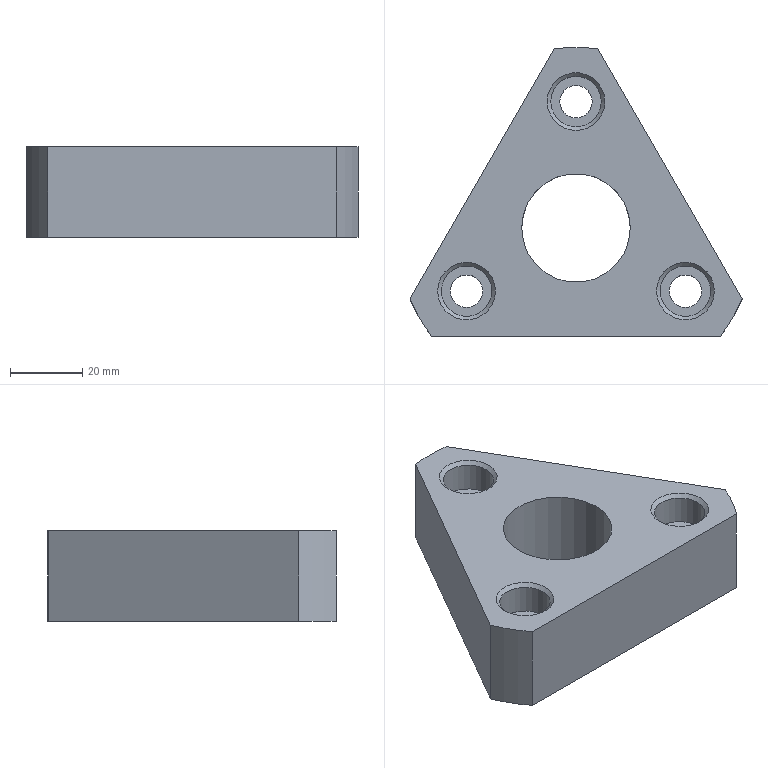Part | NX | 1 solid | 21 faces | box 91.962 x 80 x 25 mm | volume 87413 mm3 | cylinder 10 | plane 8 | cone 3 | commonest cylinder face diameters 9 x3 14 x3 100 x3 30.1 x1
STEP:
#1=CARTESIAN_POINT('',(-4.5,25.,-25.));
#2=VERTEX_POINT('',#1);
#3=CARTESIAN_POINT('',(0.,25.,-25.));
#4=DIRECTION('',(0.,0.,1.));
#5=DIRECTION('',(-1.,0.,0.));
#6=AXIS2_PLACEMENT_3D('',#3,#4,#5);
#7=CIRCLE('',#6,4.5);
#8=EDGE_CURVE('',#2,#2,#7,.T.);
#9=ORIENTED_EDGE('',*,*,#8,.F.);
#10=EDGE_LOOP('',(#9));
#11=FACE_BOUND('',#10,.T.);
#12=CARTESIAN_POINT('',(-4.5,25.,-9.));
#13=VERTEX_POINT('',#12);
#14=CARTESIAN_POINT('',(0.,25.,-9.));
#15=DIRECTION('',(0.,0.,1.));
#16=DIRECTION('',(-1.,0.,0.));
#17=AXIS2_PLACEMENT_3D('',#14,#15,#16);
#18=CIRCLE('',#17,4.5);
#19=EDGE_CURVE('',#13,#13,#18,.F.);
#20=ORIENTED_EDGE('',*,*,#19,.F.);
#21=EDGE_LOOP('',(#20));
#22=FACE_BOUND('',#21,.T.);
#23=CARTESIAN_POINT('',(0.,25.,-25.));
#24=DIRECTION('',(0.,0.,1.));
#25=DIRECTION('',(-1.,0.,0.));
#26=AXIS2_PLACEMENT_3D('',#23,#24,#25);
#27=CYLINDRICAL_SURFACE('',#26,4.5);
#28=ADVANCED_FACE('',(#11,#22),#27,.F.);
#29=CARTESIAN_POINT('',(-34.811,-27.5,-25.));
#30=VERTEX_POINT('',#29);
#31=CARTESIAN_POINT('',(-30.311,-27.5,-25.));
#32=DIRECTION('',(0.,0.,1.));
#33=DIRECTION('',(-1.,0.,0.));
#34=AXIS2_PLACEMENT_3D('',#31,#32,#33);
#35=CIRCLE('',#34,4.5);
#36=EDGE_CURVE('',#30,#30,#35,.T.);
#37=ORIENTED_EDGE('',*,*,#36,.F.);
#38=EDGE_LOOP('',(#37));
#39=FACE_BOUND('',#38,.T.);
#40=CARTESIAN_POINT('',(-34.811,-27.5,-9.));
#41=VERTEX_POINT('',#40);
#42=CARTESIAN_POINT('',(-30.311,-27.5,-9.));
#43=DIRECTION('',(0.,0.,1.));
#44=DIRECTION('',(-1.,0.,0.));
#45=AXIS2_PLACEMENT_3D('',#42,#43,#44);
#46=CIRCLE('',#45,4.5);
#47=EDGE_CURVE('',#41,#41,#46,.F.);
#48=ORIENTED_EDGE('',*,*,#47,.F.);
#49=EDGE_LOOP('',(#48));
#50=FACE_BOUND('',#49,.T.);
#51=CARTESIAN_POINT('',(-30.311,-27.5,-25.));
#52=DIRECTION('',(0.,0.,1.));
#53=DIRECTION('',(-1.,0.,0.));
#54=AXIS2_PLACEMENT_3D('',#51,#52,#53);
#55=CYLINDRICAL_SURFACE('',#54,4.5);
#56=ADVANCED_FACE('',(#39,#50),#55,.F.);
#57=CARTESIAN_POINT('',(25.811,-27.5,-25.));
#58=VERTEX_POINT('',#57);
#59=CARTESIAN_POINT('',(30.311,-27.5,-25.));
#60=DIRECTION('',(0.,0.,1.));
#61=DIRECTION('',(-1.,0.,0.));
#62=AXIS2_PLACEMENT_3D('',#59,#60,#61);
#63=CIRCLE('',#62,4.5);
#64=EDGE_CURVE('',#58,#58,#63,.T.);
#65=ORIENTED_EDGE('',*,*,#64,.F.);
#66=EDGE_LOOP('',(#65));
#67=FACE_BOUND('',#66,.T.);
#68=CARTESIAN_POINT('',(25.811,-27.5,-9.));
#69=VERTEX_POINT('',#68);
#70=CARTESIAN_POINT('',(30.311,-27.5,-9.));
#71=DIRECTION('',(0.,0.,1.));
#72=DIRECTION('',(-1.,0.,0.));
#73=AXIS2_PLACEMENT_3D('',#70,#71,#72);
#74=CIRCLE('',#73,4.5);
#75=EDGE_CURVE('',#69,#69,#74,.F.);
#76=ORIENTED_EDGE('',*,*,#75,.F.);
#77=EDGE_LOOP('',(#76));
#78=FACE_BOUND('',#77,.T.);
#79=CARTESIAN_POINT('',(30.311,-27.5,-25.));
#80=DIRECTION('',(0.,0.,1.));
#81=DIRECTION('',(-1.,0.,0.));
#82=AXIS2_PLACEMENT_3D('',#79,#80,#81);
#83=CYLINDRICAL_SURFACE('',#82,4.5);
#84=ADVANCED_FACE('',(#67,#78),#83,.F.);
#85=CARTESIAN_POINT('',(40.,-40.,0.));
#86=VERTEX_POINT('',#85);
#87=CARTESIAN_POINT('',(-40.,-40.,0.));
#88=VERTEX_POINT('',#87);
#89=CARTESIAN_POINT('',(40.,-40.,0.));
#90=DIRECTION('',(-1.,0.,0.));
#91=VECTOR('',#90,1000.);
#92=LINE('',#89,#91);
#93=EDGE_CURVE('',#86,#88,#92,.T.);
#94=ORIENTED_EDGE('',*,*,#93,.T.);
#95=CARTESIAN_POINT('',(-40.,-40.,-25.));
#96=VERTEX_POINT('',#95);
#97=CARTESIAN_POINT('',(-40.,-40.,-25.));
#98=DIRECTION('',(0.,0.,1.));
#99=VECTOR('',#98,1000.);
#100=LINE('',#97,#99);
#101=EDGE_CURVE('',#96,#88,#100,.T.);
#102=ORIENTED_EDGE('',*,*,#101,.F.);
#103=CARTESIAN_POINT('',(40.,-40.,-25.));
#104=VERTEX_POINT('',#103);
#105=CARTESIAN_POINT('',(40.,-40.,-25.));
#106=DIRECTION('',(-1.,0.,0.));
#107=VECTOR('',#106,1000.);
#108=LINE('',#105,#107);
#109=EDGE_CURVE('',#104,#96,#108,.T.);
#110=ORIENTED_EDGE('',*,*,#109,.F.);
#111=CARTESIAN_POINT('',(40.,-40.,-25.));
#112=DIRECTION('',(0.,0.,1.));
#113=VECTOR('',#112,1000.);
#114=LINE('',#111,#113);
#115=EDGE_CURVE('',#104,#86,#114,.T.);
#116=ORIENTED_EDGE('',*,*,#115,.T.);
#117=EDGE_LOOP('',(#94,#102,#110,#116));
#118=FACE_BOUND('',#117,.T.);
#119=CARTESIAN_POINT('',(40.,-40.,-25.));
#120=DIRECTION('',(0.,1.,0.));
#121=DIRECTION('',(-1.,0.,0.));
#122=AXIS2_PLACEMENT_3D('',#119,#120,#121);
#123=PLANE('',#122);
#124=ADVANCED_FACE('',(#118),#123,.F.);
#125=CARTESIAN_POINT('',(-45.981,-29.641,0.));
#126=VERTEX_POINT('',#125);
#127=CARTESIAN_POINT('',(0.,-10.,0.));
#128=DIRECTION('',(0.,0.,-1.));
#129=DIRECTION('',(-1.,0.,0.));
#130=AXIS2_PLACEMENT_3D('',#127,#128,#129);
#131=CIRCLE('',#130,50.);
#132=EDGE_CURVE('',#88,#126,#131,.T.);
#133=ORIENTED_EDGE('',*,*,#132,.T.);
#134=CARTESIAN_POINT('',(-45.981,-29.641,-25.));
#135=VERTEX_POINT('',#134);
#136=CARTESIAN_POINT('',(-45.981,-29.641,-25.));
#137=DIRECTION('',(0.,0.,1.));
#138=VECTOR('',#137,1000.);
#139=LINE('',#136,#138);
#140=EDGE_CURVE('',#135,#126,#139,.T.);
#141=ORIENTED_EDGE('',*,*,#140,.F.);
#142=CARTESIAN_POINT('',(0.,-10.,-25.));
#143=DIRECTION('',(0.,0.,-1.));
#144=DIRECTION('',(-1.,0.,0.));
#145=AXIS2_PLACEMENT_3D('',#142,#143,#144);
#146=CIRCLE('',#145,50.);
#147=EDGE_CURVE('',#96,#135,#146,.T.);
#148=ORIENTED_EDGE('',*,*,#147,.F.);
#149=ORIENTED_EDGE('',*,*,#101,.T.);
#150=EDGE_LOOP('',(#133,#141,#148,#149));
#151=FACE_BOUND('',#150,.T.);
#152=CARTESIAN_POINT('',(0.,-10.,-25.));
#153=DIRECTION('',(0.,0.,1.));
#154=DIRECTION('',(-1.,0.,0.));
#155=AXIS2_PLACEMENT_3D('',#152,#153,#154);
#156=CYLINDRICAL_SURFACE('',#155,50.);
#157=ADVANCED_FACE('',(#151),#156,.T.);
#158=CARTESIAN_POINT('',(-5.981,39.641,0.));
#159=VERTEX_POINT('',#158);
#160=CARTESIAN_POINT('',(-45.981,-29.641,0.));
#161=DIRECTION('',(0.5,0.866,0.));
#162=VECTOR('',#161,1000.);
#163=LINE('',#160,#162);
#164=EDGE_CURVE('',#126,#159,#163,.T.);
#165=ORIENTED_EDGE('',*,*,#164,.T.);
#166=CARTESIAN_POINT('',(-5.981,39.641,-25.));
#167=VERTEX_POINT('',#166);
#168=CARTESIAN_POINT('',(-5.981,39.641,-25.));
#169=DIRECTION('',(0.,0.,1.));
#170=VECTOR('',#169,1000.);
#171=LINE('',#168,#170);
#172=EDGE_CURVE('',#167,#159,#171,.T.);
#173=ORIENTED_EDGE('',*,*,#172,.F.);
#174=CARTESIAN_POINT('',(-45.981,-29.641,-25.));
#175=DIRECTION('',(0.5,0.866,0.));
#176=VECTOR('',#175,1000.);
#177=LINE('',#174,#176);
#178=EDGE_CURVE('',#135,#167,#177,.T.);
#179=ORIENTED_EDGE('',*,*,#178,.F.);
#180=ORIENTED_EDGE('',*,*,#140,.T.);
#181=EDGE_LOOP('',(#165,#173,#179,#180));
#182=FACE_BOUND('',#181,.T.);
#183=CARTESIAN_POINT('',(-45.981,-29.641,-25.));
#184=DIRECTION('',(0.866,-0.5,0.));
#185=DIRECTION('',(0.5,0.866,0.));
#186=AXIS2_PLACEMENT_3D('',#183,#184,#185);
#187=PLANE('',#186);
#188=ADVANCED_FACE('',(#182),#187,.F.);
#189=CARTESIAN_POINT('',(5.981,39.641,0.));
#190=VERTEX_POINT('',#189);
#191=CARTESIAN_POINT('',(0.,-10.,0.));
#192=DIRECTION('',(0.,0.,-1.));
#193=DIRECTION('',(-1.,0.,0.));
#194=AXIS2_PLACEMENT_3D('',#191,#192,#193);
#195=CIRCLE('',#194,50.);
#196=EDGE_CURVE('',#159,#190,#195,.T.);
#197=ORIENTED_EDGE('',*,*,#196,.T.);
#198=CARTESIAN_POINT('',(5.981,39.641,-25.));
#199=VERTEX_POINT('',#198);
#200=CARTESIAN_POINT('',(5.981,39.641,-25.));
#201=DIRECTION('',(0.,0.,1.));
#202=VECTOR('',#201,1000.);
#203=LINE('',#200,#202);
#204=EDGE_CURVE('',#199,#190,#203,.T.);
#205=ORIENTED_EDGE('',*,*,#204,.F.);
#206=CARTESIAN_POINT('',(0.,-10.,-25.));
#207=DIRECTION('',(0.,0.,-1.));
#208=DIRECTION('',(-1.,0.,0.));
#209=AXIS2_PLACEMENT_3D('',#206,#207,#208);
#210=CIRCLE('',#209,50.);
#211=EDGE_CURVE('',#167,#199,#210,.T.);
#212=ORIENTED_EDGE('',*,*,#211,.F.);
#213=ORIENTED_EDGE('',*,*,#172,.T.);
#214=EDGE_LOOP('',(#197,#205,#212,#213));
#215=FACE_BOUND('',#214,.T.);
#216=CARTESIAN_POINT('',(0.,-10.,-25.));
#217=DIRECTION('',(0.,0.,1.));
#218=DIRECTION('',(-1.,0.,0.));
#219=AXIS2_PLACEMENT_3D('',#216,#217,#218);
#220=CYLINDRICAL_SURFACE('',#219,50.);
#221=ADVANCED_FACE('',(#215),#220,.T.);
#222=CARTESIAN_POINT('',(45.981,-29.641,0.));
#223=VERTEX_POINT('',#222);
#224=CARTESIAN_POINT('',(5.981,39.641,0.));
#225=DIRECTION('',(0.5,-0.866,0.));
#226=VECTOR('',#225,1000.);
#227=LINE('',#224,#226);
#228=EDGE_CURVE('',#190,#223,#227,.T.);
#229=ORIENTED_EDGE('',*,*,#228,.T.);
#230=CARTESIAN_POINT('',(45.981,-29.641,-25.));
#231=VERTEX_POINT('',#230);
#232=CARTESIAN_POINT('',(45.981,-29.641,-25.));
#233=DIRECTION('',(0.,0.,1.));
#234=VECTOR('',#233,1000.);
#235=LINE('',#232,#234);
#236=EDGE_CURVE('',#231,#223,#235,.T.);
#237=ORIENTED_EDGE('',*,*,#236,.F.);
#238=CARTESIAN_POINT('',(5.981,39.641,-25.));
#239=DIRECTION('',(0.5,-0.866,0.));
#240=VECTOR('',#239,1000.);
#241=LINE('',#238,#240);
#242=EDGE_CURVE('',#199,#231,#241,.T.);
#243=ORIENTED_EDGE('',*,*,#242,.F.);
#244=ORIENTED_EDGE('',*,*,#204,.T.);
#245=EDGE_LOOP('',(#229,#237,#243,#244));
#246=FACE_BOUND('',#245,.T.);
#247=CARTESIAN_POINT('',(5.981,39.641,-25.));
#248=DIRECTION('',(-0.866,-0.5,0.));
#249=DIRECTION('',(0.5,-0.866,0.));
#250=AXIS2_PLACEMENT_3D('',#247,#248,#249);
#251=PLANE('',#250);
#252=ADVANCED_FACE('',(#246),#251,.F.);
#253=CARTESIAN_POINT('',(15.05,-10.,-25.));
#254=VERTEX_POINT('',#253);
#255=CARTESIAN_POINT('',(0.,-10.,-25.));
#256=DIRECTION('',(0.,0.,-1.));
#257=DIRECTION('',(1.,0.,0.));
#258=AXIS2_PLACEMENT_3D('',#255,#256,#257);
#259=CIRCLE('',#258,15.05);
#260=EDGE_CURVE('',#254,#254,#259,.F.);
#261=ORIENTED_EDGE('',*,*,#260,.F.);
#262=EDGE_LOOP('',(#261));
#263=FACE_BOUND('',#262,.T.);
#264=CARTESIAN_POINT('',(15.05,-10.,0.));
#265=VERTEX_POINT('',#264);
#266=CARTESIAN_POINT('',(0.,-10.,0.));
#267=DIRECTION('',(0.,0.,-1.));
#268=DIRECTION('',(1.,0.,0.));
#269=AXIS2_PLACEMENT_3D('',#266,#267,#268);
#270=CIRCLE('',#269,15.05);
#271=EDGE_CURVE('',#265,#265,#270,.F.);
#272=ORIENTED_EDGE('',*,*,#271,.T.);
#273=EDGE_LOOP('',(#272));
#274=FACE_BOUND('',#273,.T.);
#275=CARTESIAN_POINT('',(0.,-10.,-25.));
#276=DIRECTION('',(0.,0.,1.));
#277=DIRECTION('',(-1.,0.,0.));
#278=AXIS2_PLACEMENT_3D('',#275,#276,#277);
#279=CYLINDRICAL_SURFACE('',#278,15.05);
#280=ADVANCED_FACE('',(#263,#274),#279,.F.);
#281=CARTESIAN_POINT('',(0.,-10.,0.));
#282=DIRECTION('',(0.,0.,-1.));
#283=DIRECTION('',(-1.,0.,0.));
#284=AXIS2_PLACEMENT_3D('',#281,#282,#283);
#285=CIRCLE('',#284,50.);
#286=EDGE_CURVE('',#223,#86,#285,.T.);
#287=ORIENTED_EDGE('',*,*,#286,.T.);
#288=ORIENTED_EDGE('',*,*,#115,.F.);
#289=CARTESIAN_POINT('',(0.,-10.,-25.));
#290=DIRECTION('',(0.,0.,-1.));
#291=DIRECTION('',(-1.,0.,0.));
#292=AXIS2_PLACEMENT_3D('',#289,#290,#291);
#293=CIRCLE('',#292,50.);
#294=EDGE_CURVE('',#231,#104,#293,.T.);
#295=ORIENTED_EDGE('',*,*,#294,.F.);
#296=ORIENTED_EDGE('',*,*,#236,.T.);
#297=EDGE_LOOP('',(#287,#288,#295,#296));
#298=FACE_BOUND('',#297,.T.);
#299=CARTESIAN_POINT('',(0.,-10.,-25.));
#300=DIRECTION('',(0.,0.,1.));
#301=DIRECTION('',(-1.,0.,0.));
#302=AXIS2_PLACEMENT_3D('',#299,#300,#301);
#303=CYLINDRICAL_SURFACE('',#302,50.);
#304=ADVANCED_FACE('',(#298),#303,.T.);
#305=ORIENTED_EDGE('',*,*,#109,.T.);
#306=ORIENTED_EDGE('',*,*,#147,.T.);
#307=ORIENTED_EDGE('',*,*,#178,.T.);
#308=ORIENTED_EDGE('',*,*,#211,.T.);
#309=ORIENTED_EDGE('',*,*,#242,.T.);
#310=ORIENTED_EDGE('',*,*,#294,.T.);
#311=EDGE_LOOP('',(#305,#306,#307,#308,#309,#310));
#312=FACE_BOUND('',#311,.T.);
#313=ORIENTED_EDGE('',*,*,#36,.T.);
#314=EDGE_LOOP('',(#313));
#315=FACE_BOUND('',#314,.T.);
#316=ORIENTED_EDGE('',*,*,#8,.T.);
#317=EDGE_LOOP('',(#316));
#318=FACE_BOUND('',#317,.T.);
#319=ORIENTED_EDGE('',*,*,#260,.T.);
#320=EDGE_LOOP('',(#319));
#321=FACE_BOUND('',#320,.T.);
#322=ORIENTED_EDGE('',*,*,#64,.T.);
#323=EDGE_LOOP('',(#322));
#324=FACE_BOUND('',#323,.T.);
#325=CARTESIAN_POINT('',(0.,-10.,-25.));
#326=DIRECTION('',(0.,0.,-1.));
#327=DIRECTION('',(1.,0.,0.));
#328=AXIS2_PLACEMENT_3D('',#325,#326,#327);
#329=PLANE('',#328);
#330=ADVANCED_FACE('',(#312,#315,#318,#321,#324),#329,.T.);
#331=CARTESIAN_POINT('',(22.311,-27.5,0.));
#332=VERTEX_POINT('',#331);
#333=CARTESIAN_POINT('',(30.311,-27.5,0.));
#334=DIRECTION('',(0.,0.,-1.));
#335=DIRECTION('',(-1.,0.,0.));
#336=AXIS2_PLACEMENT_3D('',#333,#334,#335);
#337=CIRCLE('',#336,8.);
#338=EDGE_CURVE('',#332,#332,#337,.T.);
#339=ORIENTED_EDGE('',*,*,#338,.T.);
#340=EDGE_LOOP('',(#339));
#341=FACE_BOUND('',#340,.T.);
#342=CARTESIAN_POINT('',(-38.311,-27.5,0.));
#343=VERTEX_POINT('',#342);
#344=CARTESIAN_POINT('',(-30.311,-27.5,0.));
#345=DIRECTION('',(0.,0.,-1.));
#346=DIRECTION('',(-1.,0.,0.));
#347=AXIS2_PLACEMENT_3D('',#344,#345,#346);
#348=CIRCLE('',#347,8.);
#349=EDGE_CURVE('',#343,#343,#348,.T.);
#350=ORIENTED_EDGE('',*,*,#349,.T.);
#351=EDGE_LOOP('',(#350));
#352=FACE_BOUND('',#351,.T.);
#353=CARTESIAN_POINT('',(-8.,25.,0.));
#354=VERTEX_POINT('',#353);
#355=CARTESIAN_POINT('',(0.,25.,0.));
#356=DIRECTION('',(0.,0.,-1.));
#357=DIRECTION('',(-1.,0.,0.));
#358=AXIS2_PLACEMENT_3D('',#355,#356,#357);
#359=CIRCLE('',#358,8.);
#360=EDGE_CURVE('',#354,#354,#359,.T.);
#361=ORIENTED_EDGE('',*,*,#360,.T.);
#362=EDGE_LOOP('',(#361));
#363=FACE_BOUND('',#362,.T.);
#364=ORIENTED_EDGE('',*,*,#93,.F.);
#365=ORIENTED_EDGE('',*,*,#286,.F.);
#366=ORIENTED_EDGE('',*,*,#228,.F.);
#367=ORIENTED_EDGE('',*,*,#196,.F.);
#368=ORIENTED_EDGE('',*,*,#164,.F.);
#369=ORIENTED_EDGE('',*,*,#132,.F.);
#370=EDGE_LOOP('',(#364,#365,#366,#367,#368,#369));
#371=FACE_BOUND('',#370,.T.);
#372=ORIENTED_EDGE('',*,*,#271,.F.);
#373=EDGE_LOOP('',(#372));
#374=FACE_BOUND('',#373,.T.);
#375=CARTESIAN_POINT('',(0.,-10.,0.));
#376=DIRECTION('',(0.,0.,-1.));
#377=DIRECTION('',(1.,0.,0.));
#378=AXIS2_PLACEMENT_3D('',#375,#376,#377);
#379=PLANE('',#378);
#380=ADVANCED_FACE('',(#341,#352,#363,#371,#374),#379,.F.);
#381=CARTESIAN_POINT('',(23.311,-27.5,-9.));
#382=VERTEX_POINT('',#381);
#383=CARTESIAN_POINT('',(30.311,-27.5,-9.));
#384=DIRECTION('',(0.,0.,1.));
#385=DIRECTION('',(-1.,0.,0.));
#386=AXIS2_PLACEMENT_3D('',#383,#384,#385);
#387=CIRCLE('',#386,7.);
#388=EDGE_CURVE('',#382,#382,#387,.F.);
#389=ORIENTED_EDGE('',*,*,#388,.F.);
#390=EDGE_LOOP('',(#389));
#391=FACE_BOUND('',#390,.T.);
#392=ORIENTED_EDGE('',*,*,#75,.T.);
#393=EDGE_LOOP('',(#392));
#394=FACE_BOUND('',#393,.T.);
#395=CARTESIAN_POINT('',(30.311,-27.5,-9.));
#396=DIRECTION('',(0.,0.,1.));
#397=DIRECTION('',(-1.,0.,0.));
#398=AXIS2_PLACEMENT_3D('',#395,#396,#397);
#399=PLANE('',#398);
#400=ADVANCED_FACE('',(#391,#394),#399,.T.);
#401=CARTESIAN_POINT('',(23.311,-27.5,-1.));
#402=VERTEX_POINT('',#401);
#403=CARTESIAN_POINT('',(30.311,-27.5,-1.));
#404=DIRECTION('',(0.,0.,-1.));
#405=DIRECTION('',(-1.,0.,0.));
#406=AXIS2_PLACEMENT_3D('',#403,#404,#405);
#407=CIRCLE('',#406,7.);
#408=EDGE_CURVE('',#402,#402,#407,.F.);
#409=ORIENTED_EDGE('',*,*,#408,.T.);
#410=EDGE_LOOP('',(#409));
#411=FACE_BOUND('',#410,.T.);
#412=ORIENTED_EDGE('',*,*,#388,.T.);
#413=EDGE_LOOP('',(#412));
#414=FACE_BOUND('',#413,.T.);
#415=CARTESIAN_POINT('',(30.311,-27.5,-9.));
#416=DIRECTION('',(0.,0.,1.));
#417=DIRECTION('',(-1.,0.,0.));
#418=AXIS2_PLACEMENT_3D('',#415,#416,#417);
#419=CYLINDRICAL_SURFACE('',#418,7.);
#420=ADVANCED_FACE('',(#411,#414),#419,.F.);
#421=CARTESIAN_POINT('',(-7.,25.,-9.));
#422=VERTEX_POINT('',#421);
#423=CARTESIAN_POINT('',(0.,25.,-9.));
#424=DIRECTION('',(0.,0.,1.));
#425=DIRECTION('',(-1.,0.,0.));
#426=AXIS2_PLACEMENT_3D('',#423,#424,#425);
#427=CIRCLE('',#426,7.);
#428=EDGE_CURVE('',#422,#422,#427,.F.);
#429=ORIENTED_EDGE('',*,*,#428,.F.);
#430=EDGE_LOOP('',(#429));
#431=FACE_BOUND('',#430,.T.);
#432=ORIENTED_EDGE('',*,*,#19,.T.);
#433=EDGE_LOOP('',(#432));
#434=FACE_BOUND('',#433,.T.);
#435=CARTESIAN_POINT('',(0.,25.,-9.));
#436=DIRECTION('',(0.,0.,1.));
#437=DIRECTION('',(-1.,0.,0.));
#438=AXIS2_PLACEMENT_3D('',#435,#436,#437);
#439=PLANE('',#438);
#440=ADVANCED_FACE('',(#431,#434),#439,.T.);
#441=CARTESIAN_POINT('',(-7.,25.,-1.));
#442=VERTEX_POINT('',#441);
#443=CARTESIAN_POINT('',(0.,25.,-1.));
#444=DIRECTION('',(0.,0.,-1.));
#445=DIRECTION('',(-1.,0.,0.));
#446=AXIS2_PLACEMENT_3D('',#443,#444,#445);
#447=CIRCLE('',#446,7.);
#448=EDGE_CURVE('',#442,#442,#447,.F.);
#449=ORIENTED_EDGE('',*,*,#448,.T.);
#450=EDGE_LOOP('',(#449));
#451=FACE_BOUND('',#450,.T.);
#452=ORIENTED_EDGE('',*,*,#428,.T.);
#453=EDGE_LOOP('',(#452));
#454=FACE_BOUND('',#453,.T.);
#455=CARTESIAN_POINT('',(0.,25.,-9.));
#456=DIRECTION('',(0.,0.,1.));
#457=DIRECTION('',(-1.,0.,0.));
#458=AXIS2_PLACEMENT_3D('',#455,#456,#457);
#459=CYLINDRICAL_SURFACE('',#458,7.);
#460=ADVANCED_FACE('',(#451,#454),#459,.F.);
#461=CARTESIAN_POINT('',(-37.311,-27.5,-9.));
#462=VERTEX_POINT('',#461);
#463=CARTESIAN_POINT('',(-30.311,-27.5,-9.));
#464=DIRECTION('',(0.,0.,1.));
#465=DIRECTION('',(-1.,0.,0.));
#466=AXIS2_PLACEMENT_3D('',#463,#464,#465);
#467=CIRCLE('',#466,7.);
#468=EDGE_CURVE('',#462,#462,#467,.F.);
#469=ORIENTED_EDGE('',*,*,#468,.F.);
#470=EDGE_LOOP('',(#469));
#471=FACE_BOUND('',#470,.T.);
#472=ORIENTED_EDGE('',*,*,#47,.T.);
#473=EDGE_LOOP('',(#472));
#474=FACE_BOUND('',#473,.T.);
#475=CARTESIAN_POINT('',(-30.311,-27.5,-9.));
#476=DIRECTION('',(0.,0.,1.));
#477=DIRECTION('',(-1.,0.,0.));
#478=AXIS2_PLACEMENT_3D('',#475,#476,#477);
#479=PLANE('',#478);
#480=ADVANCED_FACE('',(#471,#474),#479,.T.);
#481=CARTESIAN_POINT('',(-37.311,-27.5,-1.));
#482=VERTEX_POINT('',#481);
#483=CARTESIAN_POINT('',(-30.311,-27.5,-1.));
#484=DIRECTION('',(0.,0.,-1.));
#485=DIRECTION('',(-1.,0.,0.));
#486=AXIS2_PLACEMENT_3D('',#483,#484,#485);
#487=CIRCLE('',#486,7.);
#488=EDGE_CURVE('',#482,#482,#487,.F.);
#489=ORIENTED_EDGE('',*,*,#488,.T.);
#490=EDGE_LOOP('',(#489));
#491=FACE_BOUND('',#490,.T.);
#492=ORIENTED_EDGE('',*,*,#468,.T.);
#493=EDGE_LOOP('',(#492));
#494=FACE_BOUND('',#493,.T.);
#495=CARTESIAN_POINT('',(-30.311,-27.5,-9.));
#496=DIRECTION('',(0.,0.,1.));
#497=DIRECTION('',(-1.,0.,0.));
#498=AXIS2_PLACEMENT_3D('',#495,#496,#497);
#499=CYLINDRICAL_SURFACE('',#498,7.);
#500=ADVANCED_FACE('',(#491,#494),#499,.F.);
#501=ORIENTED_EDGE('',*,*,#338,.F.);
#502=EDGE_LOOP('',(#501));
#503=FACE_BOUND('',#502,.T.);
#504=ORIENTED_EDGE('',*,*,#408,.F.);
#505=EDGE_LOOP('',(#504));
#506=FACE_BOUND('',#505,.T.);
#507=CARTESIAN_POINT('',(30.311,-27.5,-1.));
#508=DIRECTION('',(0.,0.,1.));
#509=DIRECTION('',(1.,0.,0.));
#510=AXIS2_PLACEMENT_3D('',#507,#508,#509);
#511=CONICAL_SURFACE('',#510,7.,0.7854);
#512=ADVANCED_FACE('',(#503,#506),#511,.F.);
#513=ORIENTED_EDGE('',*,*,#349,.F.);
#514=EDGE_LOOP('',(#513));
#515=FACE_BOUND('',#514,.T.);
#516=ORIENTED_EDGE('',*,*,#488,.F.);
#517=EDGE_LOOP('',(#516));
#518=FACE_BOUND('',#517,.T.);
#519=CARTESIAN_POINT('',(-30.311,-27.5,-1.));
#520=DIRECTION('',(0.,0.,1.));
#521=DIRECTION('',(1.,0.,0.));
#522=AXIS2_PLACEMENT_3D('',#519,#520,#521);
#523=CONICAL_SURFACE('',#522,7.,0.7854);
#524=ADVANCED_FACE('',(#515,#518),#523,.F.);
#525=ORIENTED_EDGE('',*,*,#360,.F.);
#526=EDGE_LOOP('',(#525));
#527=FACE_BOUND('',#526,.T.);
#528=ORIENTED_EDGE('',*,*,#448,.F.);
#529=EDGE_LOOP('',(#528));
#530=FACE_BOUND('',#529,.T.);
#531=CARTESIAN_POINT('',(0.,25.,-1.));
#532=DIRECTION('',(0.,0.,1.));
#533=DIRECTION('',(1.,0.,0.));
#534=AXIS2_PLACEMENT_3D('',#531,#532,#533);
#535=CONICAL_SURFACE('',#534,7.,0.7854);
#536=ADVANCED_FACE('',(#527,#530),#535,.F.);
#537=CLOSED_SHELL('',(#28,#56,#84,#124,#157,#188,#221,#252,#280,#304,#330,#380,#400,#420,#440,#460,#480,#500,#512,#524,#536));
#538=MANIFOLD_SOLID_BREP('',#537);
#539=(LENGTH_UNIT()NAMED_UNIT(*)SI_UNIT(.MILLI.,.METRE.));
#540=UNCERTAINTY_MEASURE_WITH_UNIT(LENGTH_MEASURE(0.00001),#539,'','');
#541=(NAMED_UNIT(*)PLANE_ANGLE_UNIT()SI_UNIT($,.RADIAN.));
#542=(NAMED_UNIT(*)SI_UNIT($,.STERADIAN.)SOLID_ANGLE_UNIT());
#543=(GEOMETRIC_REPRESENTATION_CONTEXT(3)GLOBAL_UNCERTAINTY_ASSIGNED_CONTEXT((#540))GLOBAL_UNIT_ASSIGNED_CONTEXT((#539,#541,#542))REPRESENTATION_CONTEXT('',''));
#544=ADVANCED_BREP_SHAPE_REPRESENTATION('',(#538),#543);